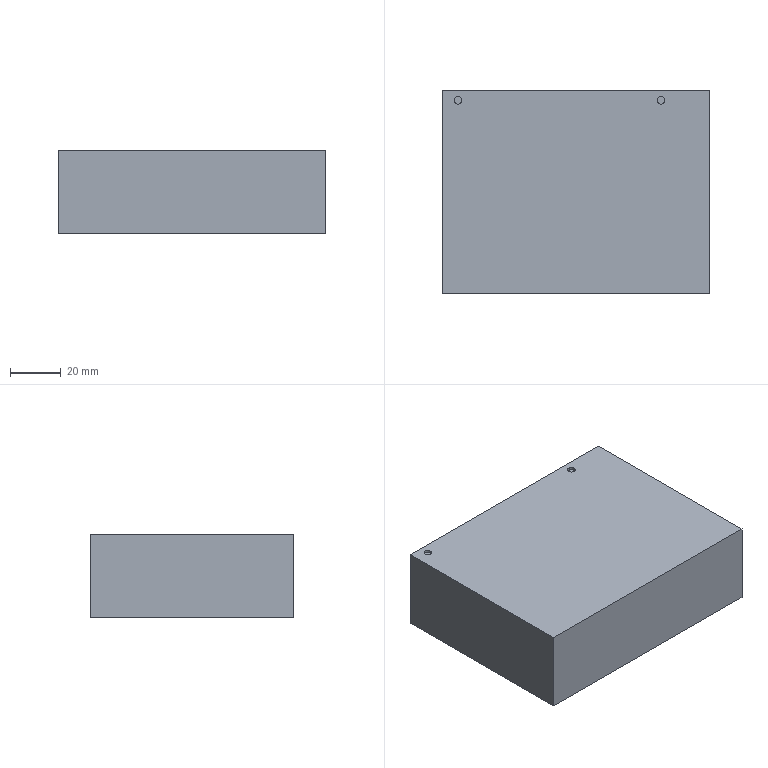Part | SolidWorks | features Extrusion 1, ICE 1, Shell 1 | 1 solid | 24 faces | box 105 x 80.181 x 33 mm | volume 28220 mm3 | plane 16 | cylinder 8 | commonest cylinder face diameters 3 x4 5 x4
STEP:
#1=CARTESIAN_POINT('',(-29.67,45.172,32.));
#2=VERTEX_POINT('',#1);
#3=CARTESIAN_POINT('',(-26.67,45.172,32.));
#4=VERTEX_POINT('',#3);
#5=CARTESIAN_POINT('',(-28.17,45.172,32.));
#6=DIRECTION('',(0.,0.,1.));
#7=DIRECTION('',(1.,0.,0.));
#8=AXIS2_PLACEMENT_3D('',#5,#6,#7);
#9=CIRCLE('',#8,1.5);
#10=EDGE_CURVE('',#2,#4,#9,.T.);
#11=ORIENTED_EDGE('',*,*,#10,.F.);
#12=CARTESIAN_POINT('',(-29.67,45.172,33.));
#13=VERTEX_POINT('',#12);
#14=CARTESIAN_POINT('',(-29.67,45.172,32.));
#15=DIRECTION('',(0.,0.,1.));
#16=VECTOR('',#15,1000.);
#17=LINE('',#14,#16);
#18=EDGE_CURVE('',#2,#13,#17,.T.);
#19=ORIENTED_EDGE('',*,*,#18,.T.);
#20=CARTESIAN_POINT('',(-26.67,45.172,33.));
#21=VERTEX_POINT('',#20);
#22=CARTESIAN_POINT('',(-28.17,45.172,33.));
#23=DIRECTION('',(0.,0.,1.));
#24=DIRECTION('',(1.,0.,0.));
#25=AXIS2_PLACEMENT_3D('',#22,#23,#24);
#26=CIRCLE('',#25,1.5);
#27=EDGE_CURVE('',#13,#21,#26,.T.);
#28=ORIENTED_EDGE('',*,*,#27,.T.);
#29=CARTESIAN_POINT('',(-26.67,45.172,32.));
#30=DIRECTION('',(0.,0.,1.));
#31=VECTOR('',#30,1000.);
#32=LINE('',#29,#31);
#33=EDGE_CURVE('',#4,#21,#32,.T.);
#34=ORIENTED_EDGE('',*,*,#33,.F.);
#35=EDGE_LOOP('',(#11,#19,#28,#34));
#36=FACE_OUTER_BOUND('',#35,.T.);
#37=CARTESIAN_POINT('',(-28.17,45.172,32.));
#38=DIRECTION('',(0.,0.,1.));
#39=DIRECTION('',(1.,0.,0.));
#40=AXIS2_PLACEMENT_3D('',#37,#38,#39);
#41=CYLINDRICAL_SURFACE('',#40,1.5);
#42=ADVANCED_FACE('',(#36),#41,.F.);
#43=CARTESIAN_POINT('',(50.33,45.172,32.));
#44=VERTEX_POINT('',#43);
#45=CARTESIAN_POINT('',(53.33,45.172,32.));
#46=VERTEX_POINT('',#45);
#47=CARTESIAN_POINT('',(51.83,45.172,32.));
#48=DIRECTION('',(0.,0.,1.));
#49=DIRECTION('',(1.,0.,0.));
#50=AXIS2_PLACEMENT_3D('',#47,#48,#49);
#51=CIRCLE('',#50,1.5);
#52=EDGE_CURVE('',#44,#46,#51,.T.);
#53=ORIENTED_EDGE('',*,*,#52,.F.);
#54=CARTESIAN_POINT('',(50.33,45.172,33.));
#55=VERTEX_POINT('',#54);
#56=CARTESIAN_POINT('',(50.33,45.172,32.));
#57=DIRECTION('',(0.,0.,1.));
#58=VECTOR('',#57,1000.);
#59=LINE('',#56,#58);
#60=EDGE_CURVE('',#44,#55,#59,.T.);
#61=ORIENTED_EDGE('',*,*,#60,.T.);
#62=CARTESIAN_POINT('',(53.33,45.172,33.));
#63=VERTEX_POINT('',#62);
#64=CARTESIAN_POINT('',(51.83,45.172,33.));
#65=DIRECTION('',(0.,0.,1.));
#66=DIRECTION('',(1.,0.,0.));
#67=AXIS2_PLACEMENT_3D('',#64,#65,#66);
#68=CIRCLE('',#67,1.5);
#69=EDGE_CURVE('',#55,#63,#68,.T.);
#70=ORIENTED_EDGE('',*,*,#69,.T.);
#71=CARTESIAN_POINT('',(53.33,45.172,32.));
#72=DIRECTION('',(0.,0.,1.));
#73=VECTOR('',#72,1000.);
#74=LINE('',#71,#73);
#75=EDGE_CURVE('',#46,#63,#74,.T.);
#76=ORIENTED_EDGE('',*,*,#75,.F.);
#77=EDGE_LOOP('',(#53,#61,#70,#76));
#78=FACE_OUTER_BOUND('',#77,.T.);
#79=CARTESIAN_POINT('',(51.83,45.172,32.));
#80=DIRECTION('',(0.,0.,1.));
#81=DIRECTION('',(1.,0.,0.));
#82=AXIS2_PLACEMENT_3D('',#79,#80,#81);
#83=CYLINDRICAL_SURFACE('',#82,1.5);
#84=ADVANCED_FACE('',(#78),#83,.F.);
#85=CARTESIAN_POINT('',(-34.17,49.172,0.));
#86=VERTEX_POINT('',#85);
#87=CARTESIAN_POINT('',(-34.17,-31.009,0.));
#88=VERTEX_POINT('',#87);
#89=CARTESIAN_POINT('',(-34.17,49.172,0.));
#90=DIRECTION('',(0.,-1.,0.));
#91=VECTOR('',#90,1000.);
#92=LINE('',#89,#91);
#93=EDGE_CURVE('',#86,#88,#92,.T.);
#94=ORIENTED_EDGE('',*,*,#93,.T.);
#95=CARTESIAN_POINT('',(-34.17,-31.009,33.));
#96=VERTEX_POINT('',#95);
#97=CARTESIAN_POINT('',(-34.17,-31.009,33.));
#98=DIRECTION('',(0.,0.,-1.));
#99=VECTOR('',#98,1000.);
#100=LINE('',#97,#99);
#101=EDGE_CURVE('',#96,#88,#100,.T.);
#102=ORIENTED_EDGE('',*,*,#101,.F.);
#103=CARTESIAN_POINT('',(-34.17,49.172,33.));
#104=VERTEX_POINT('',#103);
#105=CARTESIAN_POINT('',(-34.17,49.172,33.));
#106=DIRECTION('',(0.,-1.,0.));
#107=VECTOR('',#106,1000.);
#108=LINE('',#105,#107);
#109=EDGE_CURVE('',#104,#96,#108,.T.);
#110=ORIENTED_EDGE('',*,*,#109,.F.);
#111=CARTESIAN_POINT('',(-34.17,49.172,33.));
#112=DIRECTION('',(0.,0.,-1.));
#113=VECTOR('',#112,1000.);
#114=LINE('',#111,#113);
#115=EDGE_CURVE('',#104,#86,#114,.T.);
#116=ORIENTED_EDGE('',*,*,#115,.T.);
#117=EDGE_LOOP('',(#94,#102,#110,#116));
#118=FACE_OUTER_BOUND('',#117,.T.);
#119=CARTESIAN_POINT('',(-34.17,49.172,33.));
#120=DIRECTION('',(1.,0.,0.));
#121=DIRECTION('',(0.,0.,-1.));
#122=AXIS2_PLACEMENT_3D('',#119,#120,#121);
#123=PLANE('',#122);
#124=ADVANCED_FACE('',(#118),#123,.F.);
#125=CARTESIAN_POINT('',(70.83,-31.009,0.));
#126=VERTEX_POINT('',#125);
#127=CARTESIAN_POINT('',(-34.17,-31.009,0.));
#128=DIRECTION('',(1.,0.,0.));
#129=VECTOR('',#128,1000.);
#130=LINE('',#127,#129);
#131=EDGE_CURVE('',#88,#126,#130,.T.);
#132=ORIENTED_EDGE('',*,*,#131,.T.);
#133=CARTESIAN_POINT('',(70.83,-31.009,33.));
#134=VERTEX_POINT('',#133);
#135=CARTESIAN_POINT('',(70.83,-31.009,33.));
#136=DIRECTION('',(0.,0.,-1.));
#137=VECTOR('',#136,1000.);
#138=LINE('',#135,#137);
#139=EDGE_CURVE('',#134,#126,#138,.T.);
#140=ORIENTED_EDGE('',*,*,#139,.F.);
#141=CARTESIAN_POINT('',(-34.17,-31.009,33.));
#142=DIRECTION('',(1.,0.,0.));
#143=VECTOR('',#142,1000.);
#144=LINE('',#141,#143);
#145=EDGE_CURVE('',#96,#134,#144,.T.);
#146=ORIENTED_EDGE('',*,*,#145,.F.);
#147=ORIENTED_EDGE('',*,*,#101,.T.);
#148=EDGE_LOOP('',(#132,#140,#146,#147));
#149=FACE_OUTER_BOUND('',#148,.T.);
#150=CARTESIAN_POINT('',(-34.17,-31.009,33.));
#151=DIRECTION('',(0.,1.,0.));
#152=DIRECTION('',(0.,0.,1.));
#153=AXIS2_PLACEMENT_3D('',#150,#151,#152);
#154=PLANE('',#153);
#155=ADVANCED_FACE('',(#149),#154,.F.);
#156=CARTESIAN_POINT('',(70.83,49.172,0.));
#157=VERTEX_POINT('',#156);
#158=CARTESIAN_POINT('',(70.83,49.172,0.));
#159=DIRECTION('',(0.,1.,0.));
#160=VECTOR('',#159,1000.);
#161=LINE('',#158,#160);
#162=EDGE_CURVE('',#126,#157,#161,.T.);
#163=ORIENTED_EDGE('',*,*,#162,.T.);
#164=CARTESIAN_POINT('',(70.83,49.172,33.));
#165=VERTEX_POINT('',#164);
#166=CARTESIAN_POINT('',(70.83,49.172,33.));
#167=DIRECTION('',(0.,0.,-1.));
#168=VECTOR('',#167,1000.);
#169=LINE('',#166,#168);
#170=EDGE_CURVE('',#165,#157,#169,.T.);
#171=ORIENTED_EDGE('',*,*,#170,.F.);
#172=CARTESIAN_POINT('',(70.83,49.172,33.));
#173=DIRECTION('',(0.,1.,0.));
#174=VECTOR('',#173,1000.);
#175=LINE('',#172,#174);
#176=EDGE_CURVE('',#134,#165,#175,.T.);
#177=ORIENTED_EDGE('',*,*,#176,.F.);
#178=ORIENTED_EDGE('',*,*,#139,.T.);
#179=EDGE_LOOP('',(#163,#171,#177,#178));
#180=FACE_OUTER_BOUND('',#179,.T.);
#181=CARTESIAN_POINT('',(70.83,49.172,33.));
#182=DIRECTION('',(-1.,0.,0.));
#183=DIRECTION('',(0.,0.,1.));
#184=AXIS2_PLACEMENT_3D('',#181,#182,#183);
#185=PLANE('',#184);
#186=ADVANCED_FACE('',(#180),#185,.F.);
#187=CARTESIAN_POINT('',(-34.17,49.172,0.));
#188=DIRECTION('',(-1.,0.,0.));
#189=VECTOR('',#188,1000.);
#190=LINE('',#187,#189);
#191=EDGE_CURVE('',#157,#86,#190,.T.);
#192=ORIENTED_EDGE('',*,*,#191,.T.);
#193=ORIENTED_EDGE('',*,*,#115,.F.);
#194=CARTESIAN_POINT('',(-34.17,49.172,33.));
#195=DIRECTION('',(-1.,0.,0.));
#196=VECTOR('',#195,1000.);
#197=LINE('',#194,#196);
#198=EDGE_CURVE('',#165,#104,#197,.T.);
#199=ORIENTED_EDGE('',*,*,#198,.F.);
#200=ORIENTED_EDGE('',*,*,#170,.T.);
#201=EDGE_LOOP('',(#192,#193,#199,#200));
#202=FACE_OUTER_BOUND('',#201,.T.);
#203=CARTESIAN_POINT('',(-34.17,49.172,33.));
#204=DIRECTION('',(0.,-1.,0.));
#205=DIRECTION('',(0.,0.,-1.));
#206=AXIS2_PLACEMENT_3D('',#203,#204,#205);
#207=PLANE('',#206);
#208=ADVANCED_FACE('',(#202),#207,.F.);
#209=CARTESIAN_POINT('',(-28.17,45.172,33.));
#210=DIRECTION('',(0.,0.,1.));
#211=DIRECTION('',(1.,0.,0.));
#212=AXIS2_PLACEMENT_3D('',#209,#210,#211);
#213=CIRCLE('',#212,1.5);
#214=EDGE_CURVE('',#21,#13,#213,.T.);
#215=ORIENTED_EDGE('',*,*,#214,.F.);
#216=ORIENTED_EDGE('',*,*,#27,.F.);
#217=EDGE_LOOP('',(#215,#216));
#218=FACE_BOUND('',#217,.T.);
#219=CARTESIAN_POINT('',(51.83,45.172,33.));
#220=DIRECTION('',(0.,0.,1.));
#221=DIRECTION('',(1.,0.,0.));
#222=AXIS2_PLACEMENT_3D('',#219,#220,#221);
#223=CIRCLE('',#222,1.5);
#224=EDGE_CURVE('',#63,#55,#223,.T.);
#225=ORIENTED_EDGE('',*,*,#224,.F.);
#226=ORIENTED_EDGE('',*,*,#69,.F.);
#227=EDGE_LOOP('',(#225,#226));
#228=FACE_BOUND('',#227,.T.);
#229=ORIENTED_EDGE('',*,*,#109,.T.);
#230=ORIENTED_EDGE('',*,*,#145,.T.);
#231=ORIENTED_EDGE('',*,*,#176,.T.);
#232=ORIENTED_EDGE('',*,*,#198,.T.);
#233=EDGE_LOOP('',(#229,#230,#231,#232));
#234=FACE_OUTER_BOUND('',#233,.T.);
#235=CARTESIAN_POINT('',(0.,0.,33.));
#236=DIRECTION('',(0.,0.,1.));
#237=DIRECTION('',(1.,0.,0.));
#238=AXIS2_PLACEMENT_3D('',#235,#236,#237);
#239=PLANE('',#238);
#240=ADVANCED_FACE('',(#218,#228,#234),#239,.T.);
#241=ORIENTED_EDGE('',*,*,#93,.F.);
#242=ORIENTED_EDGE('',*,*,#191,.F.);
#243=ORIENTED_EDGE('',*,*,#162,.F.);
#244=ORIENTED_EDGE('',*,*,#131,.F.);
#245=EDGE_LOOP('',(#241,#242,#243,#244));
#246=FACE_OUTER_BOUND('',#245,.T.);
#247=CARTESIAN_POINT('',(0.,0.,0.));
#248=DIRECTION('',(0.,0.,1.));
#249=DIRECTION('',(1.,0.,0.));
#250=AXIS2_PLACEMENT_3D('',#247,#248,#249);
#251=PLANE('',#250);
#252=ADVANCED_FACE('',(#246),#251,.F.);
#253=ORIENTED_EDGE('',*,*,#60,.F.);
#254=CARTESIAN_POINT('',(51.83,45.172,32.));
#255=DIRECTION('',(0.,0.,1.));
#256=DIRECTION('',(1.,0.,0.));
#257=AXIS2_PLACEMENT_3D('',#254,#255,#256);
#258=CIRCLE('',#257,1.5);
#259=EDGE_CURVE('',#46,#44,#258,.T.);
#260=ORIENTED_EDGE('',*,*,#259,.F.);
#261=ORIENTED_EDGE('',*,*,#75,.T.);
#262=ORIENTED_EDGE('',*,*,#224,.T.);
#263=EDGE_LOOP('',(#253,#260,#261,#262));
#264=FACE_OUTER_BOUND('',#263,.T.);
#265=CARTESIAN_POINT('',(51.83,45.172,32.));
#266=DIRECTION('',(0.,0.,1.));
#267=DIRECTION('',(1.,0.,0.));
#268=AXIS2_PLACEMENT_3D('',#265,#266,#267);
#269=CYLINDRICAL_SURFACE('',#268,1.5);
#270=ADVANCED_FACE('',(#264),#269,.F.);
#271=ORIENTED_EDGE('',*,*,#259,.T.);
#272=ORIENTED_EDGE('',*,*,#52,.T.);
#273=EDGE_LOOP('',(#271,#272));
#274=FACE_OUTER_BOUND('',#273,.T.);
#275=CARTESIAN_POINT('',(51.83,45.172,32.));
#276=DIRECTION('',(0.,0.,1.));
#277=DIRECTION('',(1.,0.,0.));
#278=AXIS2_PLACEMENT_3D('',#275,#276,#277);
#279=PLANE('',#278);
#280=ADVANCED_FACE('',(#274),#279,.T.);
#281=ORIENTED_EDGE('',*,*,#18,.F.);
#282=CARTESIAN_POINT('',(-28.17,45.172,32.));
#283=DIRECTION('',(0.,0.,1.));
#284=DIRECTION('',(1.,0.,0.));
#285=AXIS2_PLACEMENT_3D('',#282,#283,#284);
#286=CIRCLE('',#285,1.5);
#287=EDGE_CURVE('',#4,#2,#286,.T.);
#288=ORIENTED_EDGE('',*,*,#287,.F.);
#289=ORIENTED_EDGE('',*,*,#33,.T.);
#290=ORIENTED_EDGE('',*,*,#214,.T.);
#291=EDGE_LOOP('',(#281,#288,#289,#290));
#292=FACE_OUTER_BOUND('',#291,.T.);
#293=CARTESIAN_POINT('',(-28.17,45.172,32.));
#294=DIRECTION('',(0.,0.,1.));
#295=DIRECTION('',(1.,0.,0.));
#296=AXIS2_PLACEMENT_3D('',#293,#294,#295);
#297=CYLINDRICAL_SURFACE('',#296,1.5);
#298=ADVANCED_FACE('',(#292),#297,.F.);
#299=ORIENTED_EDGE('',*,*,#287,.T.);
#300=ORIENTED_EDGE('',*,*,#10,.T.);
#301=EDGE_LOOP('',(#299,#300));
#302=FACE_OUTER_BOUND('',#301,.T.);
#303=CARTESIAN_POINT('',(-28.17,45.172,32.));
#304=DIRECTION('',(0.,0.,1.));
#305=DIRECTION('',(1.,0.,0.));
#306=AXIS2_PLACEMENT_3D('',#303,#304,#305);
#307=PLANE('',#306);
#308=ADVANCED_FACE('',(#302),#307,.T.);
#309=CLOSED_SHELL('',(#42,#84,#124,#155,#186,#208,#240,#252,#270,#280,#298,#308));
#310=CARTESIAN_POINT('',(-25.67,45.172,31.));
#311=VERTEX_POINT('',#310);
#312=CARTESIAN_POINT('',(-30.67,45.172,31.));
#313=VERTEX_POINT('',#312);
#314=CARTESIAN_POINT('',(-28.17,45.172,31.));
#315=DIRECTION('',(0.,0.,1.));
#316=DIRECTION('',(1.,0.,0.));
#317=AXIS2_PLACEMENT_3D('',#314,#315,#316);
#318=CIRCLE('',#317,2.5);
#319=EDGE_CURVE('',#311,#313,#318,.T.);
#320=ORIENTED_EDGE('',*,*,#319,.T.);
#321=CARTESIAN_POINT('',(-30.67,45.172,32.));
#322=VERTEX_POINT('',#321);
#323=CARTESIAN_POINT('',(-30.67,45.172,32.));
#324=DIRECTION('',(0.,0.,1.));
#325=VECTOR('',#324,1000.);
#326=LINE('',#323,#325);
#327=EDGE_CURVE('',#313,#322,#326,.T.);
#328=ORIENTED_EDGE('',*,*,#327,.T.);
#329=CARTESIAN_POINT('',(-25.67,45.172,32.));
#330=VERTEX_POINT('',#329);
#331=CARTESIAN_POINT('',(-28.17,45.172,32.));
#332=DIRECTION('',(0.,0.,1.));
#333=DIRECTION('',(1.,0.,0.));
#334=AXIS2_PLACEMENT_3D('',#331,#332,#333);
#335=CIRCLE('',#334,2.5);
#336=EDGE_CURVE('',#330,#322,#335,.T.);
#337=ORIENTED_EDGE('',*,*,#336,.F.);
#338=CARTESIAN_POINT('',(-25.67,45.172,32.));
#339=DIRECTION('',(0.,0.,1.));
#340=VECTOR('',#339,1000.);
#341=LINE('',#338,#340);
#342=EDGE_CURVE('',#311,#330,#341,.T.);
#343=ORIENTED_EDGE('',*,*,#342,.F.);
#344=EDGE_LOOP('',(#320,#328,#337,#343));
#345=FACE_OUTER_BOUND('',#344,.T.);
#346=CARTESIAN_POINT('',(-28.17,45.172,32.));
#347=DIRECTION('',(0.,0.,1.));
#348=DIRECTION('',(1.,0.,0.));
#349=AXIS2_PLACEMENT_3D('',#346,#347,#348);
#350=CYLINDRICAL_SURFACE('',#349,2.5);
#351=ADVANCED_FACE('',(#345),#350,.T.);
#352=CARTESIAN_POINT('',(54.33,45.172,31.));
#353=VERTEX_POINT('',#352);
#354=CARTESIAN_POINT('',(49.33,45.172,31.));
#355=VERTEX_POINT('',#354);
#356=CARTESIAN_POINT('',(51.83,45.172,31.));
#357=DIRECTION('',(0.,0.,1.));
#358=DIRECTION('',(1.,0.,0.));
#359=AXIS2_PLACEMENT_3D('',#356,#357,#358);
#360=CIRCLE('',#359,2.5);
#361=EDGE_CURVE('',#353,#355,#360,.T.);
#362=ORIENTED_EDGE('',*,*,#361,.T.);
#363=CARTESIAN_POINT('',(49.33,45.172,32.));
#364=VERTEX_POINT('',#363);
#365=CARTESIAN_POINT('',(49.33,45.172,32.));
#366=DIRECTION('',(0.,0.,1.));
#367=VECTOR('',#366,1000.);
#368=LINE('',#365,#367);
#369=EDGE_CURVE('',#355,#364,#368,.T.);
#370=ORIENTED_EDGE('',*,*,#369,.T.);
#371=CARTESIAN_POINT('',(54.33,45.172,32.));
#372=VERTEX_POINT('',#371);
#373=CARTESIAN_POINT('',(51.83,45.172,32.));
#374=DIRECTION('',(0.,0.,1.));
#375=DIRECTION('',(1.,0.,0.));
#376=AXIS2_PLACEMENT_3D('',#373,#374,#375);
#377=CIRCLE('',#376,2.5);
#378=EDGE_CURVE('',#372,#364,#377,.T.);
#379=ORIENTED_EDGE('',*,*,#378,.F.);
#380=CARTESIAN_POINT('',(54.33,45.172,32.));
#381=DIRECTION('',(0.,0.,1.));
#382=VECTOR('',#381,1000.);
#383=LINE('',#380,#382);
#384=EDGE_CURVE('',#353,#372,#383,.T.);
#385=ORIENTED_EDGE('',*,*,#384,.F.);
#386=EDGE_LOOP('',(#362,#370,#379,#385));
#387=FACE_OUTER_BOUND('',#386,.T.);
#388=CARTESIAN_POINT('',(51.83,45.172,32.));
#389=DIRECTION('',(0.,0.,1.));
#390=DIRECTION('',(1.,0.,0.));
#391=AXIS2_PLACEMENT_3D('',#388,#389,#390);
#392=CYLINDRICAL_SURFACE('',#391,2.5);
#393=ADVANCED_FACE('',(#387),#392,.T.);
#394=CARTESIAN_POINT('',(-33.17,48.172,1.));
#395=VERTEX_POINT('',#394);
#396=CARTESIAN_POINT('',(-33.17,-30.009,1.));
#397=VERTEX_POINT('',#396);
#398=CARTESIAN_POINT('',(-33.17,49.172,1.));
#399=DIRECTION('',(0.,-1.,0.));
#400=VECTOR('',#399,1000.);
#401=LINE('',#398,#400);
#402=EDGE_CURVE('',#395,#397,#401,.T.);
#403=ORIENTED_EDGE('',*,*,#402,.F.);
#404=CARTESIAN_POINT('',(-33.17,48.172,32.));
#405=VERTEX_POINT('',#404);
#406=CARTESIAN_POINT('',(-33.17,48.172,33.));
#407=DIRECTION('',(0.,0.,-1.));
#408=VECTOR('',#407,1000.);
#409=LINE('',#406,#408);
#410=EDGE_CURVE('',#405,#395,#409,.T.);
#411=ORIENTED_EDGE('',*,*,#410,.F.);
#412=CARTESIAN_POINT('',(-33.17,-30.009,32.));
#413=VERTEX_POINT('',#412);
#414=CARTESIAN_POINT('',(-33.17,49.172,32.));
#415=DIRECTION('',(0.,-1.,0.));
#416=VECTOR('',#415,1000.);
#417=LINE('',#414,#416);
#418=EDGE_CURVE('',#405,#413,#417,.T.);
#419=ORIENTED_EDGE('',*,*,#418,.T.);
#420=CARTESIAN_POINT('',(-33.17,-30.009,33.));
#421=DIRECTION('',(0.,0.,-1.));
#422=VECTOR('',#421,1000.);
#423=LINE('',#420,#422);
#424=EDGE_CURVE('',#413,#397,#423,.T.);
#425=ORIENTED_EDGE('',*,*,#424,.T.);
#426=EDGE_LOOP('',(#403,#411,#419,#425));
#427=FACE_OUTER_BOUND('',#426,.T.);
#428=CARTESIAN_POINT('',(-33.17,49.172,33.));
#429=DIRECTION('',(1.,0.,0.));
#430=DIRECTION('',(0.,0.,-1.));
#431=AXIS2_PLACEMENT_3D('',#428,#429,#430);
#432=PLANE('',#431);
#433=ADVANCED_FACE('',(#427),#432,.T.);
#434=CARTESIAN_POINT('',(69.83,-30.009,1.));
#435=VERTEX_POINT('',#434);
#436=CARTESIAN_POINT('',(-34.17,-30.009,1.));
#437=DIRECTION('',(1.,0.,0.));
#438=VECTOR('',#437,1000.);
#439=LINE('',#436,#438);
#440=EDGE_CURVE('',#397,#435,#439,.T.);
#441=ORIENTED_EDGE('',*,*,#440,.F.);
#442=ORIENTED_EDGE('',*,*,#424,.F.);
#443=CARTESIAN_POINT('',(69.83,-30.009,32.));
#444=VERTEX_POINT('',#443);
#445=CARTESIAN_POINT('',(-34.17,-30.009,32.));
#446=DIRECTION('',(1.,0.,0.));
#447=VECTOR('',#446,1000.);
#448=LINE('',#445,#447);
#449=EDGE_CURVE('',#413,#444,#448,.T.);
#450=ORIENTED_EDGE('',*,*,#449,.T.);
#451=CARTESIAN_POINT('',(69.83,-30.009,33.));
#452=DIRECTION('',(0.,0.,-1.));
#453=VECTOR('',#452,1000.);
#454=LINE('',#451,#453);
#455=EDGE_CURVE('',#444,#435,#454,.T.);
#456=ORIENTED_EDGE('',*,*,#455,.T.);
#457=EDGE_LOOP('',(#441,#442,#450,#456));
#458=FACE_OUTER_BOUND('',#457,.T.);
#459=CARTESIAN_POINT('',(-34.17,-30.009,33.));
#460=DIRECTION('',(0.,1.,0.));
#461=DIRECTION('',(0.,0.,1.));
#462=AXIS2_PLACEMENT_3D('',#459,#460,#461);
#463=PLANE('',#462);
#464=ADVANCED_FACE('',(#458),#463,.T.);
#465=CARTESIAN_POINT('',(69.83,48.172,1.));
#466=VERTEX_POINT('',#465);
#467=CARTESIAN_POINT('',(69.83,49.172,1.));
#468=DIRECTION('',(0.,1.,0.));
#469=VECTOR('',#468,1000.);
#470=LINE('',#467,#469);
#471=EDGE_CURVE('',#435,#466,#470,.T.);
#472=ORIENTED_EDGE('',*,*,#471,.F.);
#473=ORIENTED_EDGE('',*,*,#455,.F.);
#474=CARTESIAN_POINT('',(69.83,48.172,32.));
#475=VERTEX_POINT('',#474);
#476=CARTESIAN_POINT('',(69.83,49.172,32.));
#477=DIRECTION('',(0.,1.,0.));
#478=VECTOR('',#477,1000.);
#479=LINE('',#476,#478);
#480=EDGE_CURVE('',#444,#475,#479,.T.);
#481=ORIENTED_EDGE('',*,*,#480,.T.);
#482=CARTESIAN_POINT('',(69.83,48.172,33.));
#483=DIRECTION('',(0.,0.,-1.));
#484=VECTOR('',#483,1000.);
#485=LINE('',#482,#484);
#486=EDGE_CURVE('',#475,#466,#485,.T.);
#487=ORIENTED_EDGE('',*,*,#486,.T.);
#488=EDGE_LOOP('',(#472,#473,#481,#487));
#489=FACE_OUTER_BOUND('',#488,.T.);
#490=CARTESIAN_POINT('',(69.83,49.172,33.));
#491=DIRECTION('',(-1.,0.,0.));
#492=DIRECTION('',(0.,0.,1.));
#493=AXIS2_PLACEMENT_3D('',#490,#491,#492);
#494=PLANE('',#493);
#495=ADVANCED_FACE('',(#489),#494,.T.);
#496=CARTESIAN_POINT('',(-34.17,48.172,1.));
#497=DIRECTION('',(-1.,0.,0.));
#498=VECTOR('',#497,1000.);
#499=LINE('',#496,#498);
#500=EDGE_CURVE('',#466,#395,#499,.T.);
#501=ORIENTED_EDGE('',*,*,#500,.F.);
#502=ORIENTED_EDGE('',*,*,#486,.F.);
#503=CARTESIAN_POINT('',(-34.17,48.172,32.));
#504=DIRECTION('',(-1.,0.,0.));
#505=VECTOR('',#504,1000.);
#506=LINE('',#503,#505);
#507=EDGE_CURVE('',#475,#405,#506,.T.);
#508=ORIENTED_EDGE('',*,*,#507,.T.);
#509=ORIENTED_EDGE('',*,*,#410,.T.);
#510=EDGE_LOOP('',(#501,#502,#508,#509));
#511=FACE_OUTER_BOUND('',#510,.T.);
#512=CARTESIAN_POINT('',(-34.17,48.172,33.));
#513=DIRECTION('',(0.,-1.,0.));
#514=DIRECTION('',(0.,0.,-1.));
#515=AXIS2_PLACEMENT_3D('',#512,#513,#514);
#516=PLANE('',#515);
#517=ADVANCED_FACE('',(#511),#516,.T.);
#518=ORIENTED_EDGE('',*,*,#336,.T.);
#519=CARTESIAN_POINT('',(-28.17,45.172,32.));
#520=DIRECTION('',(0.,0.,1.));
#521=DIRECTION('',(1.,0.,0.));
#522=AXIS2_PLACEMENT_3D('',#519,#520,#521);
#523=CIRCLE('',#522,2.5);
#524=EDGE_CURVE('',#322,#330,#523,.T.);
#525=ORIENTED_EDGE('',*,*,#524,.T.);
#526=EDGE_LOOP('',(#518,#525));
#527=FACE_BOUND('',#526,.T.);
#528=ORIENTED_EDGE('',*,*,#378,.T.);
#529=CARTESIAN_POINT('',(51.83,45.172,32.));
#530=DIRECTION('',(0.,0.,1.));
#531=DIRECTION('',(1.,0.,0.));
#532=AXIS2_PLACEMENT_3D('',#529,#530,#531);
#533=CIRCLE('',#532,2.5);
#534=EDGE_CURVE('',#364,#372,#533,.T.);
#535=ORIENTED_EDGE('',*,*,#534,.T.);
#536=EDGE_LOOP('',(#528,#535));
#537=FACE_BOUND('',#536,.T.);
#538=ORIENTED_EDGE('',*,*,#418,.F.);
#539=ORIENTED_EDGE('',*,*,#507,.F.);
#540=ORIENTED_EDGE('',*,*,#480,.F.);
#541=ORIENTED_EDGE('',*,*,#449,.F.);
#542=EDGE_LOOP('',(#538,#539,#540,#541));
#543=FACE_OUTER_BOUND('',#542,.T.);
#544=CARTESIAN_POINT('',(0.,0.,32.));
#545=DIRECTION('',(0.,0.,1.));
#546=DIRECTION('',(1.,0.,0.));
#547=AXIS2_PLACEMENT_3D('',#544,#545,#546);
#548=PLANE('',#547);
#549=ADVANCED_FACE('',(#527,#537,#543),#548,.F.);
#550=ORIENTED_EDGE('',*,*,#402,.T.);
#551=ORIENTED_EDGE('',*,*,#440,.T.);
#552=ORIENTED_EDGE('',*,*,#471,.T.);
#553=ORIENTED_EDGE('',*,*,#500,.T.);
#554=EDGE_LOOP('',(#550,#551,#552,#553));
#555=FACE_OUTER_BOUND('',#554,.T.);
#556=CARTESIAN_POINT('',(0.,0.,1.));
#557=DIRECTION('',(0.,0.,1.));
#558=DIRECTION('',(1.,0.,0.));
#559=AXIS2_PLACEMENT_3D('',#556,#557,#558);
#560=PLANE('',#559);
#561=ADVANCED_FACE('',(#555),#560,.T.);
#562=ORIENTED_EDGE('',*,*,#369,.F.);
#563=CARTESIAN_POINT('',(51.83,45.172,31.));
#564=DIRECTION('',(0.,0.,1.));
#565=DIRECTION('',(1.,0.,0.));
#566=AXIS2_PLACEMENT_3D('',#563,#564,#565);
#567=CIRCLE('',#566,2.5);
#568=EDGE_CURVE('',#355,#353,#567,.T.);
#569=ORIENTED_EDGE('',*,*,#568,.T.);
#570=ORIENTED_EDGE('',*,*,#384,.T.);
#571=ORIENTED_EDGE('',*,*,#534,.F.);
#572=EDGE_LOOP('',(#562,#569,#570,#571));
#573=FACE_OUTER_BOUND('',#572,.T.);
#574=CARTESIAN_POINT('',(51.83,45.172,32.));
#575=DIRECTION('',(0.,0.,1.));
#576=DIRECTION('',(1.,0.,0.));
#577=AXIS2_PLACEMENT_3D('',#574,#575,#576);
#578=CYLINDRICAL_SURFACE('',#577,2.5);
#579=ADVANCED_FACE('',(#573),#578,.T.);
#580=ORIENTED_EDGE('',*,*,#361,.F.);
#581=ORIENTED_EDGE('',*,*,#568,.F.);
#582=EDGE_LOOP('',(#580,#581));
#583=FACE_OUTER_BOUND('',#582,.T.);
#584=CARTESIAN_POINT('',(51.83,45.172,31.));
#585=DIRECTION('',(0.,0.,1.));
#586=DIRECTION('',(1.,0.,0.));
#587=AXIS2_PLACEMENT_3D('',#584,#585,#586);
#588=PLANE('',#587);
#589=ADVANCED_FACE('',(#583),#588,.F.);
#590=ORIENTED_EDGE('',*,*,#327,.F.);
#591=CARTESIAN_POINT('',(-28.17,45.172,31.));
#592=DIRECTION('',(0.,0.,1.));
#593=DIRECTION('',(1.,0.,0.));
#594=AXIS2_PLACEMENT_3D('',#591,#592,#593);
#595=CIRCLE('',#594,2.5);
#596=EDGE_CURVE('',#313,#311,#595,.T.);
#597=ORIENTED_EDGE('',*,*,#596,.T.);
#598=ORIENTED_EDGE('',*,*,#342,.T.);
#599=ORIENTED_EDGE('',*,*,#524,.F.);
#600=EDGE_LOOP('',(#590,#597,#598,#599));
#601=FACE_OUTER_BOUND('',#600,.T.);
#602=CARTESIAN_POINT('',(-28.17,45.172,32.));
#603=DIRECTION('',(0.,0.,1.));
#604=DIRECTION('',(1.,0.,0.));
#605=AXIS2_PLACEMENT_3D('',#602,#603,#604);
#606=CYLINDRICAL_SURFACE('',#605,2.5);
#607=ADVANCED_FACE('',(#601),#606,.T.);
#608=ORIENTED_EDGE('',*,*,#319,.F.);
#609=ORIENTED_EDGE('',*,*,#596,.F.);
#610=EDGE_LOOP('',(#608,#609));
#611=FACE_OUTER_BOUND('',#610,.T.);
#612=CARTESIAN_POINT('',(-28.17,45.172,31.));
#613=DIRECTION('',(0.,0.,1.));
#614=DIRECTION('',(1.,0.,0.));
#615=AXIS2_PLACEMENT_3D('',#612,#613,#614);
#616=PLANE('',#615);
#617=ADVANCED_FACE('',(#611),#616,.F.);
#618=CLOSED_SHELL('',(#351,#393,#433,#464,#495,#517,#549,#561,#579,#589,#607,#617));
#619=ORIENTED_CLOSED_SHELL('',*,#618,.F.);
#620=BREP_WITH_VOIDS('',#309,(#619));
#621=CARTESIAN_POINT('',(0.,0.,0.));
#622=DIRECTION('',(0.,0.,1.));
#623=DIRECTION('',(1.,0.,0.));
#624=AXIS2_PLACEMENT_3D('',#621,#622,#623);
#625=(LENGTH_UNIT()NAMED_UNIT(*)SI_UNIT(.MILLI.,.METRE.));
#626=UNCERTAINTY_MEASURE_WITH_UNIT(LENGTH_MEASURE(0.00001),#625,'','');
#627=(NAMED_UNIT(*)PLANE_ANGLE_UNIT()SI_UNIT($,.RADIAN.));
#628=(NAMED_UNIT(*)SI_UNIT($,.STERADIAN.)SOLID_ANGLE_UNIT());
#629=(GEOMETRIC_REPRESENTATION_CONTEXT(3)GLOBAL_UNCERTAINTY_ASSIGNED_CONTEXT((#626))GLOBAL_UNIT_ASSIGNED_CONTEXT((#625,#627,#628))REPRESENTATION_CONTEXT('',''));
#630=ADVANCED_BREP_SHAPE_REPRESENTATION('',(#620,#624),#629);